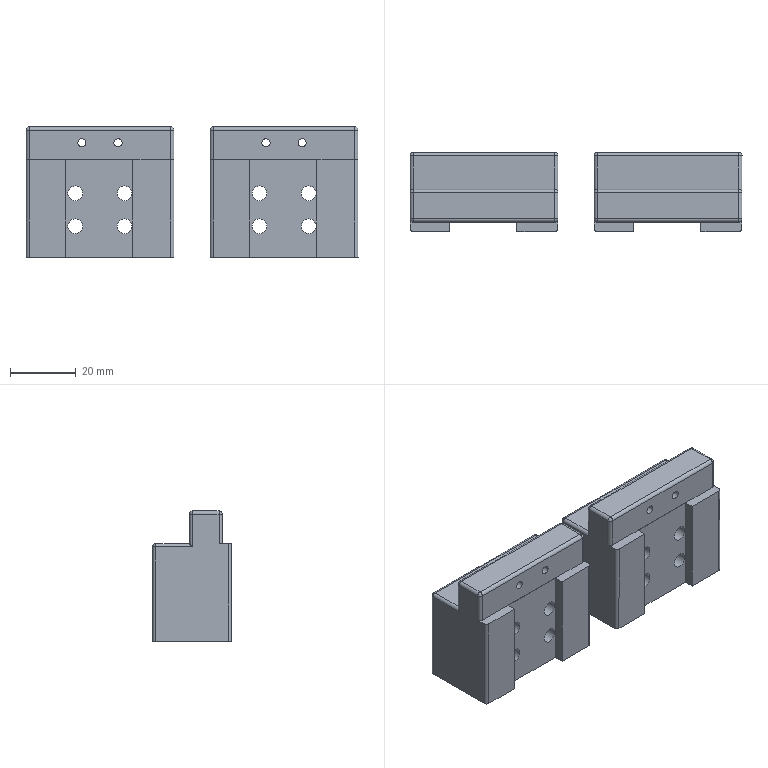Part | 3 solids | 231 faces | box 101.001 x 24.001 x 39.667 mm | volume 88901 mm3 | cylinder 105 | plane 96 | sphere 18 | cone 12 | commonest cylinder face diameters 2 x51 4.5 x12 8 x12 4 x10 2.5 x9 3 x6